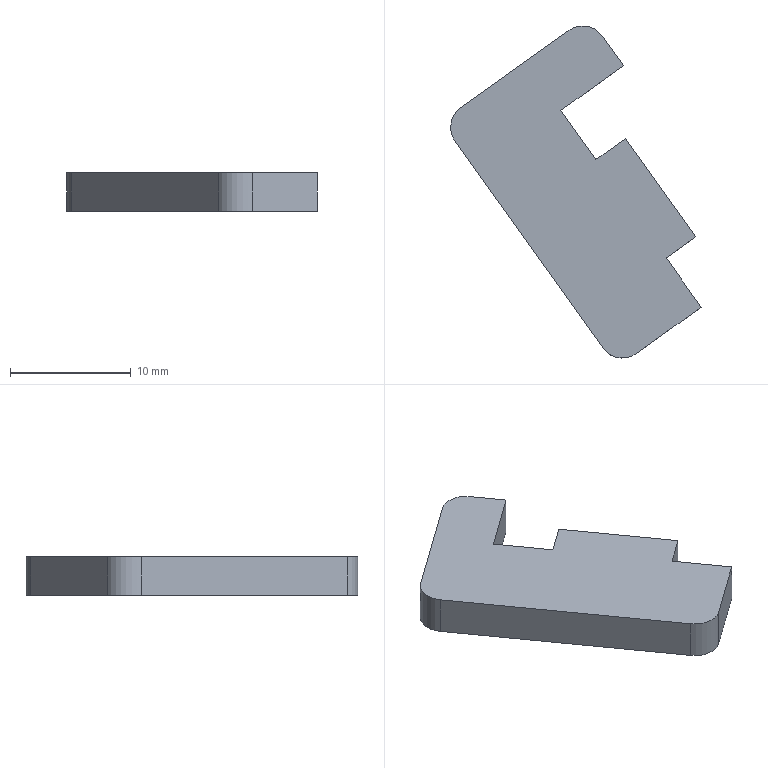Part | SolidWorks | features FlatPattern 1, SMBaseFlange 1, SheetMetal 1 | 1 solid | 15 faces | box 20.748 x 27.48 x 3.2 mm | volume 878.159 mm3 | plane 12 | cylinder 3 | commonest cylinder face diameters 4 x3
STEP:
#1=CARTESIAN_POINT('',(-145.255,-318.456,0.));
#2=VERTEX_POINT('',#1);
#3=CARTESIAN_POINT('',(-140.049,-314.733,0.));
#4=VERTEX_POINT('',#3);
#5=CARTESIAN_POINT('',(-145.255,-318.456,0.));
#6=DIRECTION('',(0.8134,0.5817,0.));
#7=VECTOR('',#6,1000.);
#8=LINE('',#5,#7);
#9=EDGE_CURVE('',#2,#4,#8,.T.);
#10=ORIENTED_EDGE('',*,*,#9,.F.);
#11=CARTESIAN_POINT('',(-145.255,-318.456,-3.2));
#12=VERTEX_POINT('',#11);
#13=CARTESIAN_POINT('',(-145.255,-318.456,-3.2));
#14=DIRECTION('',(0.,0.,1.));
#15=VECTOR('',#14,1000.);
#16=LINE('',#13,#15);
#17=EDGE_CURVE('',#12,#2,#16,.T.);
#18=ORIENTED_EDGE('',*,*,#17,.F.);
#19=CARTESIAN_POINT('',(-140.049,-314.733,-3.2));
#20=VERTEX_POINT('',#19);
#21=CARTESIAN_POINT('',(-145.255,-318.456,-3.2));
#22=DIRECTION('',(0.8134,0.5817,0.));
#23=VECTOR('',#22,1000.);
#24=LINE('',#21,#23);
#25=EDGE_CURVE('',#12,#20,#24,.T.);
#26=ORIENTED_EDGE('',*,*,#25,.T.);
#27=CARTESIAN_POINT('',(-140.049,-314.733,-3.2));
#28=DIRECTION('',(0.,0.,1.));
#29=VECTOR('',#28,1000.);
#30=LINE('',#27,#29);
#31=EDGE_CURVE('',#20,#4,#30,.T.);
#32=ORIENTED_EDGE('',*,*,#31,.T.);
#33=EDGE_LOOP('',(#10,#18,#26,#32));
#34=FACE_OUTER_BOUND('',#33,.T.);
#35=CARTESIAN_POINT('',(-145.255,-318.456,-3.2));
#36=DIRECTION('',(0.5817,-0.8134,0.));
#37=DIRECTION('',(0.8134,0.5817,0.));
#38=AXIS2_PLACEMENT_3D('',#35,#36,#37);
#39=PLANE('',#38);
#40=ADVANCED_FACE('',(#34),#39,.T.);
#41=CARTESIAN_POINT('',(-142.347,-322.523,0.));
#42=VERTEX_POINT('',#41);
#43=CARTESIAN_POINT('',(-142.347,-322.523,0.));
#44=DIRECTION('',(-0.5817,0.8134,0.));
#45=VECTOR('',#44,1000.);
#46=LINE('',#43,#45);
#47=EDGE_CURVE('',#42,#2,#46,.T.);
#48=ORIENTED_EDGE('',*,*,#47,.F.);
#49=CARTESIAN_POINT('',(-142.347,-322.523,-3.2));
#50=VERTEX_POINT('',#49);
#51=CARTESIAN_POINT('',(-142.347,-322.523,-3.2));
#52=DIRECTION('',(0.,0.,1.));
#53=VECTOR('',#52,1000.);
#54=LINE('',#51,#53);
#55=EDGE_CURVE('',#50,#42,#54,.T.);
#56=ORIENTED_EDGE('',*,*,#55,.F.);
#57=CARTESIAN_POINT('',(-142.347,-322.523,-3.2));
#58=DIRECTION('',(-0.5817,0.8134,0.));
#59=VECTOR('',#58,1000.);
#60=LINE('',#57,#59);
#61=EDGE_CURVE('',#50,#12,#60,.T.);
#62=ORIENTED_EDGE('',*,*,#61,.T.);
#63=ORIENTED_EDGE('',*,*,#17,.T.);
#64=EDGE_LOOP('',(#48,#56,#62,#63));
#65=FACE_OUTER_BOUND('',#64,.T.);
#66=CARTESIAN_POINT('',(-142.347,-322.523,-3.2));
#67=DIRECTION('',(0.8134,0.5817,0.));
#68=DIRECTION('',(-0.5817,0.8134,0.));
#69=AXIS2_PLACEMENT_3D('',#66,#67,#68);
#70=PLANE('',#69);
#71=ADVANCED_FACE('',(#65),#70,.T.);
#72=CARTESIAN_POINT('',(-139.906,-320.778,0.));
#73=VERTEX_POINT('',#72);
#74=CARTESIAN_POINT('',(-139.906,-320.778,0.));
#75=DIRECTION('',(-0.8134,-0.5817,0.));
#76=VECTOR('',#75,1000.);
#77=LINE('',#74,#76);
#78=EDGE_CURVE('',#73,#42,#77,.T.);
#79=ORIENTED_EDGE('',*,*,#78,.F.);
#80=CARTESIAN_POINT('',(-139.906,-320.778,-3.2));
#81=VERTEX_POINT('',#80);
#82=CARTESIAN_POINT('',(-139.906,-320.778,-3.2));
#83=DIRECTION('',(0.,0.,1.));
#84=VECTOR('',#83,1000.);
#85=LINE('',#82,#84);
#86=EDGE_CURVE('',#81,#73,#85,.T.);
#87=ORIENTED_EDGE('',*,*,#86,.F.);
#88=CARTESIAN_POINT('',(-139.906,-320.778,-3.2));
#89=DIRECTION('',(-0.8134,-0.5817,0.));
#90=VECTOR('',#89,1000.);
#91=LINE('',#88,#90);
#92=EDGE_CURVE('',#81,#50,#91,.T.);
#93=ORIENTED_EDGE('',*,*,#92,.T.);
#94=ORIENTED_EDGE('',*,*,#55,.T.);
#95=EDGE_LOOP('',(#79,#87,#93,#94));
#96=FACE_OUTER_BOUND('',#95,.T.);
#97=CARTESIAN_POINT('',(-139.906,-320.778,-3.2));
#98=DIRECTION('',(-0.5817,0.8134,0.));
#99=DIRECTION('',(-0.8134,-0.5817,0.));
#100=AXIS2_PLACEMENT_3D('',#97,#98,#99);
#101=PLANE('',#100);
#102=ADVANCED_FACE('',(#96),#101,.T.);
#103=CARTESIAN_POINT('',(-134.089,-328.912,0.));
#104=VERTEX_POINT('',#103);
#105=CARTESIAN_POINT('',(-134.089,-328.912,0.));
#106=DIRECTION('',(-0.5817,0.8134,0.));
#107=VECTOR('',#106,1000.);
#108=LINE('',#105,#107);
#109=EDGE_CURVE('',#104,#73,#108,.T.);
#110=ORIENTED_EDGE('',*,*,#109,.F.);
#111=CARTESIAN_POINT('',(-134.089,-328.912,-3.2));
#112=VERTEX_POINT('',#111);
#113=CARTESIAN_POINT('',(-134.089,-328.912,-3.2));
#114=DIRECTION('',(0.,0.,1.));
#115=VECTOR('',#114,1000.);
#116=LINE('',#113,#115);
#117=EDGE_CURVE('',#112,#104,#116,.T.);
#118=ORIENTED_EDGE('',*,*,#117,.F.);
#119=CARTESIAN_POINT('',(-134.089,-328.912,-3.2));
#120=DIRECTION('',(-0.5817,0.8134,0.));
#121=VECTOR('',#120,1000.);
#122=LINE('',#119,#121);
#123=EDGE_CURVE('',#112,#81,#122,.T.);
#124=ORIENTED_EDGE('',*,*,#123,.T.);
#125=ORIENTED_EDGE('',*,*,#86,.T.);
#126=EDGE_LOOP('',(#110,#118,#124,#125));
#127=FACE_OUTER_BOUND('',#126,.T.);
#128=CARTESIAN_POINT('',(-134.089,-328.912,-3.2));
#129=DIRECTION('',(0.8134,0.5817,0.));
#130=DIRECTION('',(-0.5817,0.8134,0.));
#131=AXIS2_PLACEMENT_3D('',#128,#129,#130);
#132=PLANE('',#131);
#133=ADVANCED_FACE('',(#127),#132,.T.);
#134=CARTESIAN_POINT('',(-136.53,-330.657,0.));
#135=VERTEX_POINT('',#134);
#136=CARTESIAN_POINT('',(-136.53,-330.657,0.));
#137=DIRECTION('',(0.8134,0.5817,0.));
#138=VECTOR('',#137,1000.);
#139=LINE('',#136,#138);
#140=EDGE_CURVE('',#135,#104,#139,.T.);
#141=ORIENTED_EDGE('',*,*,#140,.F.);
#142=CARTESIAN_POINT('',(-136.53,-330.657,-3.2));
#143=VERTEX_POINT('',#142);
#144=CARTESIAN_POINT('',(-136.53,-330.657,-3.2));
#145=DIRECTION('',(0.,0.,1.));
#146=VECTOR('',#145,1000.);
#147=LINE('',#144,#146);
#148=EDGE_CURVE('',#143,#135,#147,.T.);
#149=ORIENTED_EDGE('',*,*,#148,.F.);
#150=CARTESIAN_POINT('',(-136.53,-330.657,-3.2));
#151=DIRECTION('',(0.8134,0.5817,0.));
#152=VECTOR('',#151,1000.);
#153=LINE('',#150,#152);
#154=EDGE_CURVE('',#143,#112,#153,.T.);
#155=ORIENTED_EDGE('',*,*,#154,.T.);
#156=ORIENTED_EDGE('',*,*,#117,.T.);
#157=EDGE_LOOP('',(#141,#149,#155,#156));
#158=FACE_OUTER_BOUND('',#157,.T.);
#159=CARTESIAN_POINT('',(-136.53,-330.657,-3.2));
#160=DIRECTION('',(0.5817,-0.8134,0.));
#161=DIRECTION('',(0.8134,0.5817,0.));
#162=AXIS2_PLACEMENT_3D('',#159,#160,#161);
#163=PLANE('',#162);
#164=ADVANCED_FACE('',(#158),#163,.T.);
#165=CARTESIAN_POINT('',(-133.621,-334.724,0.));
#166=VERTEX_POINT('',#165);
#167=CARTESIAN_POINT('',(-133.621,-334.724,0.));
#168=DIRECTION('',(-0.5817,0.8134,0.));
#169=VECTOR('',#168,1000.);
#170=LINE('',#167,#169);
#171=EDGE_CURVE('',#166,#135,#170,.T.);
#172=ORIENTED_EDGE('',*,*,#171,.F.);
#173=CARTESIAN_POINT('',(-133.621,-334.724,-3.2));
#174=VERTEX_POINT('',#173);
#175=CARTESIAN_POINT('',(-133.621,-334.724,-3.2));
#176=DIRECTION('',(0.,0.,1.));
#177=VECTOR('',#176,1000.);
#178=LINE('',#175,#177);
#179=EDGE_CURVE('',#174,#166,#178,.T.);
#180=ORIENTED_EDGE('',*,*,#179,.F.);
#181=CARTESIAN_POINT('',(-133.621,-334.724,-3.2));
#182=DIRECTION('',(-0.5817,0.8134,0.));
#183=VECTOR('',#182,1000.);
#184=LINE('',#181,#183);
#185=EDGE_CURVE('',#174,#143,#184,.T.);
#186=ORIENTED_EDGE('',*,*,#185,.T.);
#187=ORIENTED_EDGE('',*,*,#148,.T.);
#188=EDGE_LOOP('',(#172,#180,#186,#187));
#189=FACE_OUTER_BOUND('',#188,.T.);
#190=CARTESIAN_POINT('',(-133.621,-334.724,-3.2));
#191=DIRECTION('',(0.8134,0.5817,0.));
#192=DIRECTION('',(-0.5817,0.8134,0.));
#193=AXIS2_PLACEMENT_3D('',#190,#191,#192);
#194=PLANE('',#193);
#195=ADVANCED_FACE('',(#189),#194,.T.);
#196=CARTESIAN_POINT('',(-138.99,-338.563,0.));
#197=VERTEX_POINT('',#196);
#198=CARTESIAN_POINT('',(-138.99,-338.563,0.));
#199=DIRECTION('',(0.8134,0.5817,0.));
#200=VECTOR('',#199,1000.);
#201=LINE('',#198,#200);
#202=EDGE_CURVE('',#197,#166,#201,.T.);
#203=ORIENTED_EDGE('',*,*,#202,.F.);
#204=CARTESIAN_POINT('',(-138.99,-338.563,-3.2));
#205=VERTEX_POINT('',#204);
#206=CARTESIAN_POINT('',(-138.99,-338.563,-3.2));
#207=DIRECTION('',(0.,0.,1.));
#208=VECTOR('',#207,1000.);
#209=LINE('',#206,#208);
#210=EDGE_CURVE('',#205,#197,#209,.T.);
#211=ORIENTED_EDGE('',*,*,#210,.F.);
#212=CARTESIAN_POINT('',(-138.99,-338.563,-3.2));
#213=DIRECTION('',(0.8134,0.5817,0.));
#214=VECTOR('',#213,1000.);
#215=LINE('',#212,#214);
#216=EDGE_CURVE('',#205,#174,#215,.T.);
#217=ORIENTED_EDGE('',*,*,#216,.T.);
#218=ORIENTED_EDGE('',*,*,#179,.T.);
#219=EDGE_LOOP('',(#203,#211,#217,#218));
#220=FACE_OUTER_BOUND('',#219,.T.);
#221=CARTESIAN_POINT('',(-138.99,-338.563,-3.2));
#222=DIRECTION('',(0.5817,-0.8134,0.));
#223=DIRECTION('',(0.8134,0.5817,0.));
#224=AXIS2_PLACEMENT_3D('',#221,#222,#223);
#225=PLANE('',#224);
#226=ADVANCED_FACE('',(#220),#225,.T.);
#227=CARTESIAN_POINT('',(-141.78,-338.1,0.));
#228=VERTEX_POINT('',#227);
#229=CARTESIAN_POINT('',(-140.153,-336.936,0.));
#230=DIRECTION('',(0.,0.,1.));
#231=DIRECTION('',(-1.,0.,0.));
#232=AXIS2_PLACEMENT_3D('',#229,#230,#231);
#233=CIRCLE('',#232,2.);
#234=EDGE_CURVE('',#228,#197,#233,.T.);
#235=ORIENTED_EDGE('',*,*,#234,.F.);
#236=CARTESIAN_POINT('',(-141.78,-338.1,-3.2));
#237=VERTEX_POINT('',#236);
#238=CARTESIAN_POINT('',(-141.78,-338.1,-3.2));
#239=DIRECTION('',(0.,0.,1.));
#240=VECTOR('',#239,1000.);
#241=LINE('',#238,#240);
#242=EDGE_CURVE('',#237,#228,#241,.T.);
#243=ORIENTED_EDGE('',*,*,#242,.F.);
#244=CARTESIAN_POINT('',(-140.153,-336.936,-3.2));
#245=DIRECTION('',(0.,0.,1.));
#246=DIRECTION('',(-1.,0.,0.));
#247=AXIS2_PLACEMENT_3D('',#244,#245,#246);
#248=CIRCLE('',#247,2.);
#249=EDGE_CURVE('',#237,#205,#248,.T.);
#250=ORIENTED_EDGE('',*,*,#249,.T.);
#251=ORIENTED_EDGE('',*,*,#210,.T.);
#252=EDGE_LOOP('',(#235,#243,#250,#251));
#253=FACE_OUTER_BOUND('',#252,.T.);
#254=CARTESIAN_POINT('',(-140.153,-336.936,-3.2));
#255=DIRECTION('',(0.,0.,1.));
#256=DIRECTION('',(1.,0.,0.));
#257=AXIS2_PLACEMENT_3D('',#254,#255,#256);
#258=CYLINDRICAL_SURFACE('',#257,2.);
#259=ADVANCED_FACE('',(#253),#258,.T.);
#260=CARTESIAN_POINT('',(-153.996,-321.018,0.));
#261=VERTEX_POINT('',#260);
#262=CARTESIAN_POINT('',(-153.996,-321.018,0.));
#263=DIRECTION('',(0.5817,-0.8134,0.));
#264=VECTOR('',#263,1000.);
#265=LINE('',#262,#264);
#266=EDGE_CURVE('',#261,#228,#265,.T.);
#267=ORIENTED_EDGE('',*,*,#266,.F.);
#268=CARTESIAN_POINT('',(-153.996,-321.018,-3.2));
#269=VERTEX_POINT('',#268);
#270=CARTESIAN_POINT('',(-153.996,-321.018,-3.2));
#271=DIRECTION('',(0.,0.,1.));
#272=VECTOR('',#271,1000.);
#273=LINE('',#270,#272);
#274=EDGE_CURVE('',#269,#261,#273,.T.);
#275=ORIENTED_EDGE('',*,*,#274,.F.);
#276=CARTESIAN_POINT('',(-153.996,-321.018,-3.2));
#277=DIRECTION('',(0.5817,-0.8134,0.));
#278=VECTOR('',#277,1000.);
#279=LINE('',#276,#278);
#280=EDGE_CURVE('',#269,#237,#279,.T.);
#281=ORIENTED_EDGE('',*,*,#280,.T.);
#282=ORIENTED_EDGE('',*,*,#242,.T.);
#283=EDGE_LOOP('',(#267,#275,#281,#282));
#284=FACE_OUTER_BOUND('',#283,.T.);
#285=CARTESIAN_POINT('',(-153.996,-321.018,-3.2));
#286=DIRECTION('',(-0.8134,-0.5817,0.));
#287=DIRECTION('',(0.5817,-0.8134,0.));
#288=AXIS2_PLACEMENT_3D('',#285,#286,#287);
#289=PLANE('',#288);
#290=ADVANCED_FACE('',(#284),#289,.T.);
#291=CARTESIAN_POINT('',(-153.532,-318.228,0.));
#292=VERTEX_POINT('',#291);
#293=CARTESIAN_POINT('',(-152.369,-319.855,0.));
#294=DIRECTION('',(0.,0.,1.));
#295=DIRECTION('',(1.,0.,0.));
#296=AXIS2_PLACEMENT_3D('',#293,#294,#295);
#297=CIRCLE('',#296,2.);
#298=EDGE_CURVE('',#292,#261,#297,.T.);
#299=ORIENTED_EDGE('',*,*,#298,.F.);
#300=CARTESIAN_POINT('',(-153.532,-318.228,-3.2));
#301=VERTEX_POINT('',#300);
#302=CARTESIAN_POINT('',(-153.532,-318.228,-3.2));
#303=DIRECTION('',(0.,0.,1.));
#304=VECTOR('',#303,1000.);
#305=LINE('',#302,#304);
#306=EDGE_CURVE('',#301,#292,#305,.T.);
#307=ORIENTED_EDGE('',*,*,#306,.F.);
#308=CARTESIAN_POINT('',(-152.369,-319.855,-3.2));
#309=DIRECTION('',(0.,0.,1.));
#310=DIRECTION('',(1.,0.,0.));
#311=AXIS2_PLACEMENT_3D('',#308,#309,#310);
#312=CIRCLE('',#311,2.);
#313=EDGE_CURVE('',#301,#269,#312,.T.);
#314=ORIENTED_EDGE('',*,*,#313,.T.);
#315=ORIENTED_EDGE('',*,*,#274,.T.);
#316=EDGE_LOOP('',(#299,#307,#314,#315));
#317=FACE_OUTER_BOUND('',#316,.T.);
#318=CARTESIAN_POINT('',(-152.369,-319.855,-3.2));
#319=DIRECTION('',(0.,0.,1.));
#320=DIRECTION('',(1.,0.,0.));
#321=AXIS2_PLACEMENT_3D('',#318,#319,#320);
#322=CYLINDRICAL_SURFACE('',#321,2.);
#323=ADVANCED_FACE('',(#317),#322,.T.);
#324=CARTESIAN_POINT('',(-144.585,-311.829,0.));
#325=VERTEX_POINT('',#324);
#326=CARTESIAN_POINT('',(-144.585,-311.829,0.));
#327=DIRECTION('',(-0.8134,-0.5817,0.));
#328=VECTOR('',#327,1000.);
#329=LINE('',#326,#328);
#330=EDGE_CURVE('',#325,#292,#329,.T.);
#331=ORIENTED_EDGE('',*,*,#330,.F.);
#332=CARTESIAN_POINT('',(-144.585,-311.829,-3.2));
#333=VERTEX_POINT('',#332);
#334=CARTESIAN_POINT('',(-144.585,-311.829,-3.2));
#335=DIRECTION('',(0.,0.,1.));
#336=VECTOR('',#335,1000.);
#337=LINE('',#334,#336);
#338=EDGE_CURVE('',#333,#325,#337,.T.);
#339=ORIENTED_EDGE('',*,*,#338,.F.);
#340=CARTESIAN_POINT('',(-144.585,-311.829,-3.2));
#341=DIRECTION('',(-0.8134,-0.5817,0.));
#342=VECTOR('',#341,1000.);
#343=LINE('',#340,#342);
#344=EDGE_CURVE('',#333,#301,#343,.T.);
#345=ORIENTED_EDGE('',*,*,#344,.T.);
#346=ORIENTED_EDGE('',*,*,#306,.T.);
#347=EDGE_LOOP('',(#331,#339,#345,#346));
#348=FACE_OUTER_BOUND('',#347,.T.);
#349=CARTESIAN_POINT('',(-144.585,-311.829,-3.2));
#350=DIRECTION('',(-0.5817,0.8134,0.));
#351=DIRECTION('',(-0.8134,-0.5817,0.));
#352=AXIS2_PLACEMENT_3D('',#349,#350,#351);
#353=PLANE('',#352);
#354=ADVANCED_FACE('',(#348),#353,.T.);
#355=CARTESIAN_POINT('',(-141.794,-312.293,0.));
#356=VERTEX_POINT('',#355);
#357=CARTESIAN_POINT('',(-143.421,-313.456,0.));
#358=DIRECTION('',(0.,0.,1.));
#359=DIRECTION('',(-1.,0.,0.));
#360=AXIS2_PLACEMENT_3D('',#357,#358,#359);
#361=CIRCLE('',#360,2.);
#362=EDGE_CURVE('',#356,#325,#361,.T.);
#363=ORIENTED_EDGE('',*,*,#362,.F.);
#364=CARTESIAN_POINT('',(-141.794,-312.293,-3.2));
#365=VERTEX_POINT('',#364);
#366=CARTESIAN_POINT('',(-141.794,-312.293,-3.2));
#367=DIRECTION('',(0.,0.,1.));
#368=VECTOR('',#367,1000.);
#369=LINE('',#366,#368);
#370=EDGE_CURVE('',#365,#356,#369,.T.);
#371=ORIENTED_EDGE('',*,*,#370,.F.);
#372=CARTESIAN_POINT('',(-143.421,-313.456,-3.2));
#373=DIRECTION('',(0.,0.,1.));
#374=DIRECTION('',(-1.,0.,0.));
#375=AXIS2_PLACEMENT_3D('',#372,#373,#374);
#376=CIRCLE('',#375,2.);
#377=EDGE_CURVE('',#365,#333,#376,.T.);
#378=ORIENTED_EDGE('',*,*,#377,.T.);
#379=ORIENTED_EDGE('',*,*,#338,.T.);
#380=EDGE_LOOP('',(#363,#371,#378,#379));
#381=FACE_OUTER_BOUND('',#380,.T.);
#382=CARTESIAN_POINT('',(-143.421,-313.456,-3.2));
#383=DIRECTION('',(0.,0.,1.));
#384=DIRECTION('',(1.,0.,0.));
#385=AXIS2_PLACEMENT_3D('',#382,#383,#384);
#386=CYLINDRICAL_SURFACE('',#385,2.);
#387=ADVANCED_FACE('',(#381),#386,.T.);
#388=CARTESIAN_POINT('',(-140.049,-314.733,0.));
#389=DIRECTION('',(-0.5817,0.8134,0.));
#390=VECTOR('',#389,1000.);
#391=LINE('',#388,#390);
#392=EDGE_CURVE('',#4,#356,#391,.T.);
#393=ORIENTED_EDGE('',*,*,#392,.F.);
#394=ORIENTED_EDGE('',*,*,#31,.F.);
#395=CARTESIAN_POINT('',(-140.049,-314.733,-3.2));
#396=DIRECTION('',(-0.5817,0.8134,0.));
#397=VECTOR('',#396,1000.);
#398=LINE('',#395,#397);
#399=EDGE_CURVE('',#20,#365,#398,.T.);
#400=ORIENTED_EDGE('',*,*,#399,.T.);
#401=ORIENTED_EDGE('',*,*,#370,.T.);
#402=EDGE_LOOP('',(#393,#394,#400,#401));
#403=FACE_OUTER_BOUND('',#402,.T.);
#404=CARTESIAN_POINT('',(-140.049,-314.733,-3.2));
#405=DIRECTION('',(0.8134,0.5817,0.));
#406=DIRECTION('',(-0.5817,0.8134,0.));
#407=AXIS2_PLACEMENT_3D('',#404,#405,#406);
#408=PLANE('',#407);
#409=ADVANCED_FACE('',(#403),#408,.T.);
#410=ORIENTED_EDGE('',*,*,#25,.F.);
#411=ORIENTED_EDGE('',*,*,#61,.F.);
#412=ORIENTED_EDGE('',*,*,#92,.F.);
#413=ORIENTED_EDGE('',*,*,#123,.F.);
#414=ORIENTED_EDGE('',*,*,#154,.F.);
#415=ORIENTED_EDGE('',*,*,#185,.F.);
#416=ORIENTED_EDGE('',*,*,#216,.F.);
#417=ORIENTED_EDGE('',*,*,#249,.F.);
#418=ORIENTED_EDGE('',*,*,#280,.F.);
#419=ORIENTED_EDGE('',*,*,#313,.F.);
#420=ORIENTED_EDGE('',*,*,#344,.F.);
#421=ORIENTED_EDGE('',*,*,#377,.F.);
#422=ORIENTED_EDGE('',*,*,#399,.F.);
#423=EDGE_LOOP('',(#410,#411,#412,#413,#414,#415,#416,#417,#418,#419,#420,#421,#422));
#424=FACE_OUTER_BOUND('',#423,.T.);
#425=CARTESIAN_POINT('',(-143.421,-313.456,-3.2));
#426=DIRECTION('',(0.,0.,-1.));
#427=DIRECTION('',(-1.,0.,0.));
#428=AXIS2_PLACEMENT_3D('',#425,#426,#427);
#429=PLANE('',#428);
#430=ADVANCED_FACE('',(#424),#429,.T.);
#431=ORIENTED_EDGE('',*,*,#9,.T.);
#432=ORIENTED_EDGE('',*,*,#392,.T.);
#433=ORIENTED_EDGE('',*,*,#362,.T.);
#434=ORIENTED_EDGE('',*,*,#330,.T.);
#435=ORIENTED_EDGE('',*,*,#298,.T.);
#436=ORIENTED_EDGE('',*,*,#266,.T.);
#437=ORIENTED_EDGE('',*,*,#234,.T.);
#438=ORIENTED_EDGE('',*,*,#202,.T.);
#439=ORIENTED_EDGE('',*,*,#171,.T.);
#440=ORIENTED_EDGE('',*,*,#140,.T.);
#441=ORIENTED_EDGE('',*,*,#109,.T.);
#442=ORIENTED_EDGE('',*,*,#78,.T.);
#443=ORIENTED_EDGE('',*,*,#47,.T.);
#444=EDGE_LOOP('',(#431,#432,#433,#434,#435,#436,#437,#438,#439,#440,#441,#442,#443));
#445=FACE_OUTER_BOUND('',#444,.T.);
#446=CARTESIAN_POINT('',(-143.421,-313.456,0.));
#447=DIRECTION('',(0.,0.,-1.));
#448=DIRECTION('',(-1.,0.,0.));
#449=AXIS2_PLACEMENT_3D('',#446,#447,#448);
#450=PLANE('',#449);
#451=ADVANCED_FACE('',(#445),#450,.F.);
#452=CLOSED_SHELL('',(#40,#71,#102,#133,#164,#195,#226,#259,#290,#323,#354,#387,#409,#430,#451));
#453=MANIFOLD_SOLID_BREP('',#452);
#454=CARTESIAN_POINT('',(0.,0.,0.));
#455=DIRECTION('',(0.,0.,1.));
#456=DIRECTION('',(1.,0.,0.));
#457=AXIS2_PLACEMENT_3D('',#454,#455,#456);
#458=(LENGTH_UNIT()NAMED_UNIT(*)SI_UNIT(.MILLI.,.METRE.));
#459=UNCERTAINTY_MEASURE_WITH_UNIT(LENGTH_MEASURE(0.00001),#458,'','');
#460=(NAMED_UNIT(*)PLANE_ANGLE_UNIT()SI_UNIT($,.RADIAN.));
#461=(NAMED_UNIT(*)SI_UNIT($,.STERADIAN.)SOLID_ANGLE_UNIT());
#462=(GEOMETRIC_REPRESENTATION_CONTEXT(3)GLOBAL_UNCERTAINTY_ASSIGNED_CONTEXT((#459))GLOBAL_UNIT_ASSIGNED_CONTEXT((#458,#460,#461))REPRESENTATION_CONTEXT('',''));
#463=ADVANCED_BREP_SHAPE_REPRESENTATION('',(#453,#457),#462);